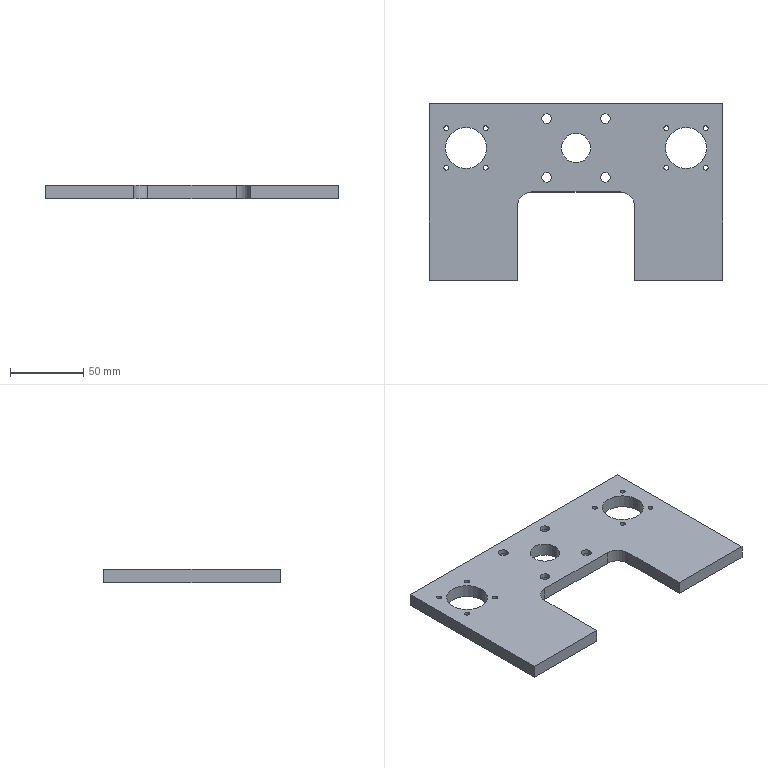Part | STEP file | X77-03211g | 1 solid | 54 faces | box 200 x 120 x 9 mm | volume 156017 mm3 | cylinder 40 | plane 14 | commonest cylinder face diameters 3.3 x16 6.6 x8 11 x8 20 x4 28 x4